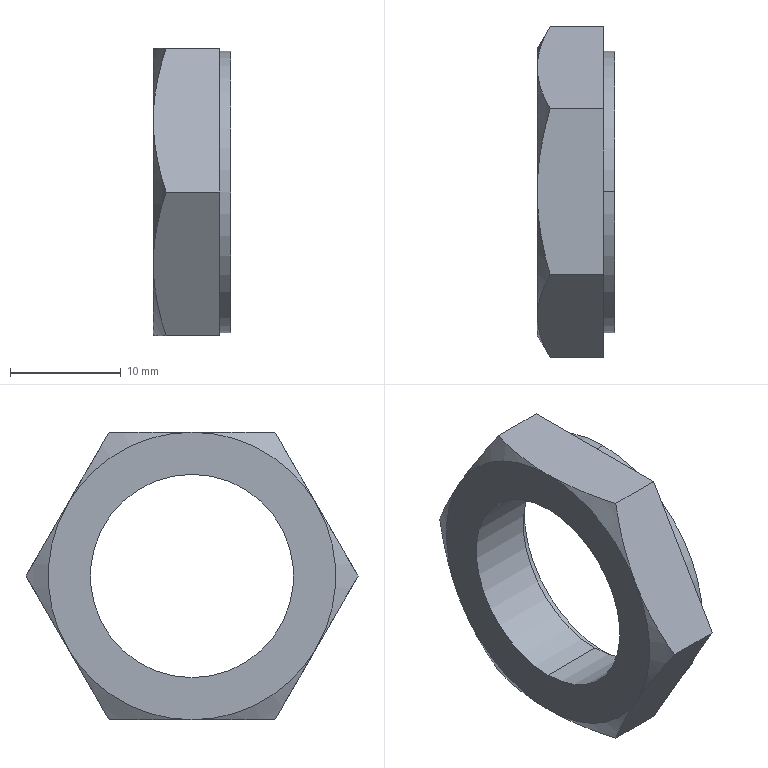Part | 1 solid | 22 faces | box 7 x 30.022 x 26 mm | volume 2098 mm3 | plane 10 | cylinder 6 | cone 6 | commonest cylinder face diameters 18.376 x2 20 x2 25.5 x2
STEP:
#1=CARTESIAN_POINT('',(7.,0.,-12.75));
#2=VERTEX_POINT('',#1);
#3=CARTESIAN_POINT('',(7.,0.,12.75));
#4=VERTEX_POINT('',#3);
#5=CARTESIAN_POINT('',(7.,0.,0.));
#6=DIRECTION('',(1.,0.,0.));
#7=DIRECTION('',(0.,0.,-1.));
#8=AXIS2_PLACEMENT_3D('',#5,#6,#7);
#9=CIRCLE('',#8,12.75);
#10=EDGE_CURVE('',#2,#4,#9,.T.);
#11=ORIENTED_EDGE('',*,*,#10,.F.);
#12=CARTESIAN_POINT('',(6.,0.,-12.75));
#13=VERTEX_POINT('',#12);
#14=CARTESIAN_POINT('',(7.,0.,-12.75));
#15=DIRECTION('',(-1.,0.,0.));
#16=VECTOR('',#15,1000.);
#17=LINE('',#14,#16);
#18=EDGE_CURVE('',#2,#13,#17,.T.);
#19=ORIENTED_EDGE('',*,*,#18,.T.);
#20=CARTESIAN_POINT('',(6.,0.,12.75));
#21=VERTEX_POINT('',#20);
#22=CARTESIAN_POINT('',(6.,0.,0.));
#23=DIRECTION('',(1.,0.,0.));
#24=DIRECTION('',(0.,0.,-1.));
#25=AXIS2_PLACEMENT_3D('',#22,#23,#24);
#26=CIRCLE('',#25,12.75);
#27=EDGE_CURVE('',#13,#21,#26,.T.);
#28=ORIENTED_EDGE('',*,*,#27,.T.);
#29=CARTESIAN_POINT('',(7.,0.,12.75));
#30=DIRECTION('',(-1.,0.,0.));
#31=VECTOR('',#30,1000.);
#32=LINE('',#29,#31);
#33=EDGE_CURVE('',#4,#21,#32,.T.);
#34=ORIENTED_EDGE('',*,*,#33,.F.);
#35=EDGE_LOOP('',(#11,#19,#28,#34));
#36=FACE_OUTER_BOUND('',#35,.T.);
#37=CARTESIAN_POINT('',(7.,0.,0.));
#38=DIRECTION('',(-1.,0.,0.));
#39=DIRECTION('',(0.,0.,1.));
#40=AXIS2_PLACEMENT_3D('',#37,#38,#39);
#41=CYLINDRICAL_SURFACE('',#40,12.75);
#42=ADVANCED_FACE('',(#36),#41,.T.);
#43=CARTESIAN_POINT('',(7.,0.,10.));
#44=VERTEX_POINT('',#43);
#45=CARTESIAN_POINT('',(7.,0.,-10.));
#46=VERTEX_POINT('',#45);
#47=CARTESIAN_POINT('',(7.,0.,0.));
#48=DIRECTION('',(1.,0.,0.));
#49=DIRECTION('',(0.,0.,-1.));
#50=AXIS2_PLACEMENT_3D('',#47,#48,#49);
#51=CIRCLE('',#50,10.);
#52=EDGE_CURVE('',#44,#46,#51,.T.);
#53=ORIENTED_EDGE('',*,*,#52,.T.);
#54=CARTESIAN_POINT('',(6.,0.,-10.));
#55=VERTEX_POINT('',#54);
#56=CARTESIAN_POINT('',(7.,0.,-10.));
#57=DIRECTION('',(-1.,0.,0.));
#58=VECTOR('',#57,1000.);
#59=LINE('',#56,#58);
#60=EDGE_CURVE('',#46,#55,#59,.T.);
#61=ORIENTED_EDGE('',*,*,#60,.T.);
#62=CARTESIAN_POINT('',(6.,0.,10.));
#63=VERTEX_POINT('',#62);
#64=CARTESIAN_POINT('',(6.,0.,0.));
#65=DIRECTION('',(-1.,0.,0.));
#66=DIRECTION('',(0.,0.,-1.));
#67=AXIS2_PLACEMENT_3D('',#64,#65,#66);
#68=CIRCLE('',#67,10.);
#69=EDGE_CURVE('',#55,#63,#68,.T.);
#70=ORIENTED_EDGE('',*,*,#69,.T.);
#71=CARTESIAN_POINT('',(7.,0.,10.));
#72=DIRECTION('',(-1.,0.,0.));
#73=VECTOR('',#72,1000.);
#74=LINE('',#71,#73);
#75=EDGE_CURVE('',#44,#63,#74,.T.);
#76=ORIENTED_EDGE('',*,*,#75,.F.);
#77=EDGE_LOOP('',(#53,#61,#70,#76));
#78=FACE_OUTER_BOUND('',#77,.T.);
#79=CARTESIAN_POINT('',(7.,0.,0.));
#80=DIRECTION('',(-1.,0.,0.));
#81=DIRECTION('',(0.,0.,1.));
#82=AXIS2_PLACEMENT_3D('',#79,#80,#81);
#83=CYLINDRICAL_SURFACE('',#82,10.);
#84=ADVANCED_FACE('',(#78),#83,.F.);
#85=CARTESIAN_POINT('',(0.,0.,9.188));
#86=VERTEX_POINT('',#85);
#87=CARTESIAN_POINT('',(0.,0.,-9.188));
#88=VERTEX_POINT('',#87);
#89=CARTESIAN_POINT('',(0.,0.,0.));
#90=DIRECTION('',(1.,0.,0.));
#91=DIRECTION('',(0.,0.,-1.));
#92=AXIS2_PLACEMENT_3D('',#89,#90,#91);
#93=CIRCLE('',#92,9.188);
#94=EDGE_CURVE('',#86,#88,#93,.T.);
#95=ORIENTED_EDGE('',*,*,#94,.F.);
#96=CARTESIAN_POINT('',(6.,0.,9.188));
#97=VERTEX_POINT('',#96);
#98=CARTESIAN_POINT('',(6.,0.,9.188));
#99=DIRECTION('',(1.,0.,0.));
#100=VECTOR('',#99,1000.);
#101=LINE('',#98,#100);
#102=EDGE_CURVE('',#86,#97,#101,.T.);
#103=ORIENTED_EDGE('',*,*,#102,.T.);
#104=CARTESIAN_POINT('',(6.,0.,-9.188));
#105=VERTEX_POINT('',#104);
#106=CARTESIAN_POINT('',(6.,0.,0.));
#107=DIRECTION('',(1.,0.,0.));
#108=DIRECTION('',(0.,0.,-1.));
#109=AXIS2_PLACEMENT_3D('',#106,#107,#108);
#110=CIRCLE('',#109,9.188);
#111=EDGE_CURVE('',#97,#105,#110,.T.);
#112=ORIENTED_EDGE('',*,*,#111,.T.);
#113=CARTESIAN_POINT('',(6.,0.,-9.188));
#114=DIRECTION('',(1.,0.,0.));
#115=VECTOR('',#114,1000.);
#116=LINE('',#113,#115);
#117=EDGE_CURVE('',#88,#105,#116,.T.);
#118=ORIENTED_EDGE('',*,*,#117,.F.);
#119=EDGE_LOOP('',(#95,#103,#112,#118));
#120=FACE_OUTER_BOUND('',#119,.T.);
#121=CARTESIAN_POINT('',(6.,0.,0.));
#122=DIRECTION('',(1.,0.,0.));
#123=DIRECTION('',(0.,0.,-1.));
#124=AXIS2_PLACEMENT_3D('',#121,#122,#123);
#125=CYLINDRICAL_SURFACE('',#124,9.188);
#126=ADVANCED_FACE('',(#120),#125,.F.);
#127=CARTESIAN_POINT('',(1.161,7.506,-13.));
#128=VERTEX_POINT('',#127);
#129=CARTESIAN_POINT('',(0.,11.258,-6.5));
#130=VERTEX_POINT('',#129);
#131=CARTESIAN_POINT('',(1.161,7.506,-13.));
#132=CARTESIAN_POINT('',(0.387,8.846,-10.678));
#133=CARTESIAN_POINT('',(0.,10.097,-8.511));
#134=CARTESIAN_POINT('',(0.,11.258,-6.5));
#135=B_SPLINE_CURVE_WITH_KNOTS('',3,(#131,#132,#133,#134),.UNSPECIFIED.,.F.,.F.,(4,4),(0.,1.),.UNSPECIFIED.);
#136=EDGE_CURVE('',#128,#130,#135,.T.);
#137=ORIENTED_EDGE('',*,*,#136,.F.);
#138=CARTESIAN_POINT('',(0.,0.,-13.));
#139=VERTEX_POINT('',#138);
#140=CARTESIAN_POINT('',(0.,0.,-13.));
#141=CARTESIAN_POINT('',(0.,2.322,-13.));
#142=CARTESIAN_POINT('',(0.387,4.824,-13.));
#143=CARTESIAN_POINT('',(1.161,7.506,-13.));
#144=B_SPLINE_CURVE_WITH_KNOTS('',3,(#140,#141,#142,#143),.UNSPECIFIED.,.F.,.F.,(4,4),(0.,1.),.UNSPECIFIED.);
#145=EDGE_CURVE('',#139,#128,#144,.T.);
#146=ORIENTED_EDGE('',*,*,#145,.F.);
#147=CARTESIAN_POINT('',(0.,0.,0.));
#148=DIRECTION('',(1.,0.,0.));
#149=DIRECTION('',(0.,0.,-1.));
#150=AXIS2_PLACEMENT_3D('',#147,#148,#149);
#151=CIRCLE('',#150,13.);
#152=EDGE_CURVE('',#139,#130,#151,.T.);
#153=ORIENTED_EDGE('',*,*,#152,.T.);
#154=EDGE_LOOP('',(#137,#146,#153));
#155=FACE_OUTER_BOUND('',#154,.T.);
#156=CARTESIAN_POINT('',(3.,0.,0.));
#157=DIRECTION('',(1.,0.,0.));
#158=DIRECTION('',(0.,0.,-1.));
#159=AXIS2_PLACEMENT_3D('',#156,#157,#158);
#160=CONICAL_SURFACE('',#159,18.196,1.047);
#161=ADVANCED_FACE('',(#155),#160,.T.);
#162=CARTESIAN_POINT('',(1.161,15.011,0.));
#163=VERTEX_POINT('',#162);
#164=CARTESIAN_POINT('',(0.,11.258,-6.5));
#165=CARTESIAN_POINT('',(0.,12.419,-4.489));
#166=CARTESIAN_POINT('',(0.387,13.67,-2.322));
#167=CARTESIAN_POINT('',(1.161,15.011,0.));
#168=B_SPLINE_CURVE_WITH_KNOTS('',3,(#164,#165,#166,#167),.UNSPECIFIED.,.F.,.F.,(4,4),(0.,1.),.UNSPECIFIED.);
#169=EDGE_CURVE('',#130,#163,#168,.T.);
#170=ORIENTED_EDGE('',*,*,#169,.F.);
#171=CARTESIAN_POINT('',(0.,11.258,6.5));
#172=VERTEX_POINT('',#171);
#173=CARTESIAN_POINT('',(0.,0.,0.));
#174=DIRECTION('',(1.,0.,0.));
#175=DIRECTION('',(0.,0.,-1.));
#176=AXIS2_PLACEMENT_3D('',#173,#174,#175);
#177=CIRCLE('',#176,13.);
#178=EDGE_CURVE('',#130,#172,#177,.T.);
#179=ORIENTED_EDGE('',*,*,#178,.T.);
#180=CARTESIAN_POINT('',(1.161,15.011,0.));
#181=CARTESIAN_POINT('',(0.387,13.67,2.322));
#182=CARTESIAN_POINT('',(0.,12.419,4.489));
#183=CARTESIAN_POINT('',(0.,11.258,6.5));
#184=B_SPLINE_CURVE_WITH_KNOTS('',3,(#180,#181,#182,#183),.UNSPECIFIED.,.F.,.F.,(4,4),(0.,1.),.UNSPECIFIED.);
#185=EDGE_CURVE('',#163,#172,#184,.T.);
#186=ORIENTED_EDGE('',*,*,#185,.F.);
#187=EDGE_LOOP('',(#170,#179,#186));
#188=FACE_OUTER_BOUND('',#187,.T.);
#189=CARTESIAN_POINT('',(3.,0.,0.));
#190=DIRECTION('',(1.,0.,0.));
#191=DIRECTION('',(0.,0.,-1.));
#192=AXIS2_PLACEMENT_3D('',#189,#190,#191);
#193=CONICAL_SURFACE('',#192,18.196,1.047);
#194=ADVANCED_FACE('',(#188),#193,.T.);
#195=CARTESIAN_POINT('',(1.161,7.506,13.));
#196=VERTEX_POINT('',#195);
#197=CARTESIAN_POINT('',(0.,11.258,6.5));
#198=CARTESIAN_POINT('',(0.,10.097,8.511));
#199=CARTESIAN_POINT('',(0.387,8.846,10.678));
#200=CARTESIAN_POINT('',(1.161,7.506,13.));
#201=B_SPLINE_CURVE_WITH_KNOTS('',3,(#197,#198,#199,#200),.UNSPECIFIED.,.F.,.F.,(4,4),(0.,1.),.UNSPECIFIED.);
#202=EDGE_CURVE('',#172,#196,#201,.T.);
#203=ORIENTED_EDGE('',*,*,#202,.F.);
#204=CARTESIAN_POINT('',(0.,0.,13.));
#205=VERTEX_POINT('',#204);
#206=CARTESIAN_POINT('',(0.,0.,0.));
#207=DIRECTION('',(1.,0.,0.));
#208=DIRECTION('',(0.,0.,-1.));
#209=AXIS2_PLACEMENT_3D('',#206,#207,#208);
#210=CIRCLE('',#209,13.);
#211=EDGE_CURVE('',#172,#205,#210,.T.);
#212=ORIENTED_EDGE('',*,*,#211,.T.);
#213=CARTESIAN_POINT('',(1.161,7.506,13.));
#214=CARTESIAN_POINT('',(0.387,4.824,13.));
#215=CARTESIAN_POINT('',(0.,2.322,13.));
#216=CARTESIAN_POINT('',(0.,0.,13.));
#217=B_SPLINE_CURVE_WITH_KNOTS('',3,(#213,#214,#215,#216),.UNSPECIFIED.,.F.,.F.,(4,4),(0.,1.),.UNSPECIFIED.);
#218=EDGE_CURVE('',#196,#205,#217,.T.);
#219=ORIENTED_EDGE('',*,*,#218,.F.);
#220=EDGE_LOOP('',(#203,#212,#219));
#221=FACE_OUTER_BOUND('',#220,.T.);
#222=CARTESIAN_POINT('',(3.,0.,0.));
#223=DIRECTION('',(1.,0.,0.));
#224=DIRECTION('',(0.,0.,-1.));
#225=AXIS2_PLACEMENT_3D('',#222,#223,#224);
#226=CONICAL_SURFACE('',#225,18.196,1.047);
#227=ADVANCED_FACE('',(#221),#226,.T.);
#228=CARTESIAN_POINT('',(1.161,-7.506,-13.));
#229=VERTEX_POINT('',#228);
#230=CARTESIAN_POINT('',(1.161,-7.506,-13.));
#231=CARTESIAN_POINT('',(0.387,-4.824,-13.));
#232=CARTESIAN_POINT('',(0.,-2.322,-13.));
#233=CARTESIAN_POINT('',(0.,0.,-13.));
#234=B_SPLINE_CURVE_WITH_KNOTS('',3,(#230,#231,#232,#233),.UNSPECIFIED.,.F.,.F.,(4,4),(0.,1.),.UNSPECIFIED.);
#235=EDGE_CURVE('',#229,#139,#234,.T.);
#236=ORIENTED_EDGE('',*,*,#235,.F.);
#237=CARTESIAN_POINT('',(0.,-11.258,-6.5));
#238=VERTEX_POINT('',#237);
#239=CARTESIAN_POINT('',(0.,-11.258,-6.5));
#240=CARTESIAN_POINT('',(0.,-10.097,-8.511));
#241=CARTESIAN_POINT('',(0.387,-8.846,-10.678));
#242=CARTESIAN_POINT('',(1.161,-7.506,-13.));
#243=B_SPLINE_CURVE_WITH_KNOTS('',3,(#239,#240,#241,#242),.UNSPECIFIED.,.F.,.F.,(4,4),(0.,1.),.UNSPECIFIED.);
#244=EDGE_CURVE('',#238,#229,#243,.T.);
#245=ORIENTED_EDGE('',*,*,#244,.F.);
#246=CARTESIAN_POINT('',(0.,0.,0.));
#247=DIRECTION('',(1.,0.,0.));
#248=DIRECTION('',(0.,0.,-1.));
#249=AXIS2_PLACEMENT_3D('',#246,#247,#248);
#250=CIRCLE('',#249,13.);
#251=EDGE_CURVE('',#238,#139,#250,.T.);
#252=ORIENTED_EDGE('',*,*,#251,.T.);
#253=EDGE_LOOP('',(#236,#245,#252));
#254=FACE_OUTER_BOUND('',#253,.T.);
#255=CARTESIAN_POINT('',(3.,0.,0.));
#256=DIRECTION('',(1.,0.,0.));
#257=DIRECTION('',(0.,0.,-1.));
#258=AXIS2_PLACEMENT_3D('',#255,#256,#257);
#259=CONICAL_SURFACE('',#258,18.196,1.047);
#260=ADVANCED_FACE('',(#254),#259,.T.);
#261=CARTESIAN_POINT('',(1.161,-7.506,13.));
#262=VERTEX_POINT('',#261);
#263=CARTESIAN_POINT('',(0.,0.,13.));
#264=CARTESIAN_POINT('',(0.,-2.322,13.));
#265=CARTESIAN_POINT('',(0.387,-4.824,13.));
#266=CARTESIAN_POINT('',(1.161,-7.506,13.));
#267=B_SPLINE_CURVE_WITH_KNOTS('',3,(#263,#264,#265,#266),.UNSPECIFIED.,.F.,.F.,(4,4),(0.,1.),.UNSPECIFIED.);
#268=EDGE_CURVE('',#205,#262,#267,.T.);
#269=ORIENTED_EDGE('',*,*,#268,.F.);
#270=CARTESIAN_POINT('',(0.,-11.258,6.5));
#271=VERTEX_POINT('',#270);
#272=CARTESIAN_POINT('',(0.,0.,0.));
#273=DIRECTION('',(1.,0.,0.));
#274=DIRECTION('',(0.,0.,-1.));
#275=AXIS2_PLACEMENT_3D('',#272,#273,#274);
#276=CIRCLE('',#275,13.);
#277=EDGE_CURVE('',#205,#271,#276,.T.);
#278=ORIENTED_EDGE('',*,*,#277,.T.);
#279=CARTESIAN_POINT('',(1.161,-7.506,13.));
#280=CARTESIAN_POINT('',(0.387,-8.846,10.678));
#281=CARTESIAN_POINT('',(0.,-10.097,8.511));
#282=CARTESIAN_POINT('',(0.,-11.258,6.5));
#283=B_SPLINE_CURVE_WITH_KNOTS('',3,(#279,#280,#281,#282),.UNSPECIFIED.,.F.,.F.,(4,4),(0.,1.),.UNSPECIFIED.);
#284=EDGE_CURVE('',#262,#271,#283,.T.);
#285=ORIENTED_EDGE('',*,*,#284,.F.);
#286=EDGE_LOOP('',(#269,#278,#285));
#287=FACE_OUTER_BOUND('',#286,.T.);
#288=CARTESIAN_POINT('',(3.,0.,0.));
#289=DIRECTION('',(1.,0.,0.));
#290=DIRECTION('',(0.,0.,-1.));
#291=AXIS2_PLACEMENT_3D('',#288,#289,#290);
#292=CONICAL_SURFACE('',#291,18.196,1.047);
#293=ADVANCED_FACE('',(#287),#292,.T.);
#294=CARTESIAN_POINT('',(6.,0.,0.));
#295=DIRECTION('',(1.,0.,0.));
#296=DIRECTION('',(0.,0.,-1.));
#297=AXIS2_PLACEMENT_3D('',#294,#295,#296);
#298=CIRCLE('',#297,9.188);
#299=EDGE_CURVE('',#105,#97,#298,.T.);
#300=ORIENTED_EDGE('',*,*,#299,.F.);
#301=ORIENTED_EDGE('',*,*,#111,.F.);
#302=EDGE_LOOP('',(#300,#301));
#303=FACE_BOUND('',#302,.T.);
#304=CARTESIAN_POINT('',(6.,0.,0.));
#305=DIRECTION('',(-1.,0.,0.));
#306=DIRECTION('',(0.,0.,-1.));
#307=AXIS2_PLACEMENT_3D('',#304,#305,#306);
#308=CIRCLE('',#307,10.);
#309=EDGE_CURVE('',#63,#55,#308,.T.);
#310=ORIENTED_EDGE('',*,*,#309,.F.);
#311=ORIENTED_EDGE('',*,*,#69,.F.);
#312=EDGE_LOOP('',(#310,#311));
#313=FACE_OUTER_BOUND('',#312,.T.);
#314=CARTESIAN_POINT('',(6.,9.188,0.));
#315=DIRECTION('',(1.,0.,0.));
#316=DIRECTION('',(0.,1.,0.));
#317=AXIS2_PLACEMENT_3D('',#314,#315,#316);
#318=PLANE('',#317);
#319=ADVANCED_FACE('',(#303,#313),#318,.T.);
#320=CARTESIAN_POINT('',(0.,0.,0.));
#321=DIRECTION('',(1.,0.,0.));
#322=DIRECTION('',(0.,0.,-1.));
#323=AXIS2_PLACEMENT_3D('',#320,#321,#322);
#324=CIRCLE('',#323,9.188);
#325=EDGE_CURVE('',#88,#86,#324,.T.);
#326=ORIENTED_EDGE('',*,*,#325,.T.);
#327=ORIENTED_EDGE('',*,*,#94,.T.);
#328=EDGE_LOOP('',(#326,#327));
#329=FACE_BOUND('',#328,.T.);
#330=ORIENTED_EDGE('',*,*,#152,.F.);
#331=ORIENTED_EDGE('',*,*,#251,.F.);
#332=CARTESIAN_POINT('',(0.,0.,0.));
#333=DIRECTION('',(1.,0.,0.));
#334=DIRECTION('',(0.,0.,-1.));
#335=AXIS2_PLACEMENT_3D('',#332,#333,#334);
#336=CIRCLE('',#335,13.);
#337=EDGE_CURVE('',#271,#238,#336,.T.);
#338=ORIENTED_EDGE('',*,*,#337,.F.);
#339=ORIENTED_EDGE('',*,*,#277,.F.);
#340=ORIENTED_EDGE('',*,*,#211,.F.);
#341=ORIENTED_EDGE('',*,*,#178,.F.);
#342=EDGE_LOOP('',(#330,#331,#338,#339,#340,#341));
#343=FACE_OUTER_BOUND('',#342,.T.);
#344=CARTESIAN_POINT('',(0.,13.,0.));
#345=DIRECTION('',(-1.,0.,0.));
#346=DIRECTION('',(0.,0.,1.));
#347=AXIS2_PLACEMENT_3D('',#344,#345,#346);
#348=PLANE('',#347);
#349=ADVANCED_FACE('',(#329,#343),#348,.T.);
#350=ORIENTED_EDGE('',*,*,#102,.F.);
#351=ORIENTED_EDGE('',*,*,#325,.F.);
#352=ORIENTED_EDGE('',*,*,#117,.T.);
#353=ORIENTED_EDGE('',*,*,#299,.T.);
#354=EDGE_LOOP('',(#350,#351,#352,#353));
#355=FACE_OUTER_BOUND('',#354,.T.);
#356=CARTESIAN_POINT('',(6.,0.,0.));
#357=DIRECTION('',(1.,0.,0.));
#358=DIRECTION('',(0.,0.,-1.));
#359=AXIS2_PLACEMENT_3D('',#356,#357,#358);
#360=CYLINDRICAL_SURFACE('',#359,9.188);
#361=ADVANCED_FACE('',(#355),#360,.F.);
#362=CARTESIAN_POINT('',(6.,-7.506,13.));
#363=VERTEX_POINT('',#362);
#364=CARTESIAN_POINT('',(6.,7.506,13.));
#365=VERTEX_POINT('',#364);
#366=CARTESIAN_POINT('',(6.,9.188,13.));
#367=DIRECTION('',(0.,1.,0.));
#368=VECTOR('',#367,1000.);
#369=LINE('',#366,#368);
#370=EDGE_CURVE('',#363,#365,#369,.T.);
#371=ORIENTED_EDGE('',*,*,#370,.F.);
#372=CARTESIAN_POINT('',(6.,-15.011,0.));
#373=VERTEX_POINT('',#372);
#374=CARTESIAN_POINT('',(6.,-8.961,10.479));
#375=DIRECTION('',(0.,0.5,0.866));
#376=VECTOR('',#375,1000.);
#377=LINE('',#374,#376);
#378=EDGE_CURVE('',#373,#363,#377,.T.);
#379=ORIENTED_EDGE('',*,*,#378,.F.);
#380=CARTESIAN_POINT('',(6.,-7.506,-13.));
#381=VERTEX_POINT('',#380);
#382=CARTESIAN_POINT('',(6.,-8.961,-10.479));
#383=DIRECTION('',(0.,-0.5,0.866));
#384=VECTOR('',#383,1000.);
#385=LINE('',#382,#384);
#386=EDGE_CURVE('',#381,#373,#385,.T.);
#387=ORIENTED_EDGE('',*,*,#386,.F.);
#388=CARTESIAN_POINT('',(6.,7.506,-13.));
#389=VERTEX_POINT('',#388);
#390=CARTESIAN_POINT('',(6.,9.188,-13.));
#391=DIRECTION('',(0.,-1.,0.));
#392=VECTOR('',#391,1000.);
#393=LINE('',#390,#392);
#394=EDGE_CURVE('',#389,#381,#393,.T.);
#395=ORIENTED_EDGE('',*,*,#394,.F.);
#396=CARTESIAN_POINT('',(6.,15.011,0.));
#397=VERTEX_POINT('',#396);
#398=CARTESIAN_POINT('',(6.,13.555,-2.521));
#399=DIRECTION('',(0.,-0.5,-0.866));
#400=VECTOR('',#399,1000.);
#401=LINE('',#398,#400);
#402=EDGE_CURVE('',#397,#389,#401,.T.);
#403=ORIENTED_EDGE('',*,*,#402,.F.);
#404=CARTESIAN_POINT('',(6.,13.555,2.521));
#405=DIRECTION('',(0.,0.5,-0.866));
#406=VECTOR('',#405,1000.);
#407=LINE('',#404,#406);
#408=EDGE_CURVE('',#365,#397,#407,.T.);
#409=ORIENTED_EDGE('',*,*,#408,.F.);
#410=EDGE_LOOP('',(#371,#379,#387,#395,#403,#409));
#411=FACE_OUTER_BOUND('',#410,.T.);
#412=CARTESIAN_POINT('',(6.,0.,0.));
#413=DIRECTION('',(1.,0.,0.));
#414=DIRECTION('',(0.,0.,-1.));
#415=AXIS2_PLACEMENT_3D('',#412,#413,#414);
#416=CIRCLE('',#415,12.75);
#417=EDGE_CURVE('',#21,#13,#416,.T.);
#418=ORIENTED_EDGE('',*,*,#417,.F.);
#419=ORIENTED_EDGE('',*,*,#27,.F.);
#420=EDGE_LOOP('',(#418,#419));
#421=FACE_BOUND('',#420,.T.);
#422=CARTESIAN_POINT('',(6.,9.188,0.));
#423=DIRECTION('',(1.,0.,0.));
#424=DIRECTION('',(0.,1.,0.));
#425=AXIS2_PLACEMENT_3D('',#422,#423,#424);
#426=PLANE('',#425);
#427=ADVANCED_FACE('',(#411,#421),#426,.T.);
#428=CARTESIAN_POINT('',(1.161,-15.011,0.));
#429=VERTEX_POINT('',#428);
#430=CARTESIAN_POINT('',(1.161,-15.011,0.));
#431=CARTESIAN_POINT('',(0.387,-13.67,-2.322));
#432=CARTESIAN_POINT('',(0.,-12.419,-4.489));
#433=CARTESIAN_POINT('',(0.,-11.258,-6.5));
#434=B_SPLINE_CURVE_WITH_KNOTS('',3,(#430,#431,#432,#433),.UNSPECIFIED.,.F.,.F.,(4,4),(0.,1.),.UNSPECIFIED.);
#435=EDGE_CURVE('',#429,#238,#434,.T.);
#436=ORIENTED_EDGE('',*,*,#435,.F.);
#437=CARTESIAN_POINT('',(0.,-11.258,6.5));
#438=CARTESIAN_POINT('',(0.,-12.419,4.489));
#439=CARTESIAN_POINT('',(0.387,-13.67,2.322));
#440=CARTESIAN_POINT('',(1.161,-15.011,0.));
#441=B_SPLINE_CURVE_WITH_KNOTS('',3,(#437,#438,#439,#440),.UNSPECIFIED.,.F.,.F.,(4,4),(0.,1.),.UNSPECIFIED.);
#442=EDGE_CURVE('',#271,#429,#441,.T.);
#443=ORIENTED_EDGE('',*,*,#442,.F.);
#444=ORIENTED_EDGE('',*,*,#337,.T.);
#445=EDGE_LOOP('',(#436,#443,#444));
#446=FACE_OUTER_BOUND('',#445,.T.);
#447=CARTESIAN_POINT('',(3.,0.,0.));
#448=DIRECTION('',(1.,0.,0.));
#449=DIRECTION('',(0.,0.,-1.));
#450=AXIS2_PLACEMENT_3D('',#447,#448,#449);
#451=CONICAL_SURFACE('',#450,18.196,1.047);
#452=ADVANCED_FACE('',(#446),#451,.T.);
#453=ORIENTED_EDGE('',*,*,#60,.F.);
#454=CARTESIAN_POINT('',(7.,0.,0.));
#455=DIRECTION('',(1.,0.,0.));
#456=DIRECTION('',(0.,0.,-1.));
#457=AXIS2_PLACEMENT_3D('',#454,#455,#456);
#458=CIRCLE('',#457,10.);
#459=EDGE_CURVE('',#46,#44,#458,.T.);
#460=ORIENTED_EDGE('',*,*,#459,.T.);
#461=ORIENTED_EDGE('',*,*,#75,.T.);
#462=ORIENTED_EDGE('',*,*,#309,.T.);
#463=EDGE_LOOP('',(#453,#460,#461,#462));
#464=FACE_OUTER_BOUND('',#463,.T.);
#465=CARTESIAN_POINT('',(7.,0.,0.));
#466=DIRECTION('',(-1.,0.,0.));
#467=DIRECTION('',(0.,0.,1.));
#468=AXIS2_PLACEMENT_3D('',#465,#466,#467);
#469=CYLINDRICAL_SURFACE('',#468,10.);
#470=ADVANCED_FACE('',(#464),#469,.F.);
#471=ORIENTED_EDGE('',*,*,#18,.F.);
#472=CARTESIAN_POINT('',(7.,0.,0.));
#473=DIRECTION('',(1.,0.,0.));
#474=DIRECTION('',(0.,0.,-1.));
#475=AXIS2_PLACEMENT_3D('',#472,#473,#474);
#476=CIRCLE('',#475,12.75);
#477=EDGE_CURVE('',#4,#2,#476,.T.);
#478=ORIENTED_EDGE('',*,*,#477,.F.);
#479=ORIENTED_EDGE('',*,*,#33,.T.);
#480=ORIENTED_EDGE('',*,*,#417,.T.);
#481=EDGE_LOOP('',(#471,#478,#479,#480));
#482=FACE_OUTER_BOUND('',#481,.T.);
#483=CARTESIAN_POINT('',(7.,0.,0.));
#484=DIRECTION('',(-1.,0.,0.));
#485=DIRECTION('',(0.,0.,1.));
#486=AXIS2_PLACEMENT_3D('',#483,#484,#485);
#487=CYLINDRICAL_SURFACE('',#486,12.75);
#488=ADVANCED_FACE('',(#482),#487,.T.);
#489=ORIENTED_EDGE('',*,*,#52,.F.);
#490=ORIENTED_EDGE('',*,*,#459,.F.);
#491=EDGE_LOOP('',(#489,#490));
#492=FACE_BOUND('',#491,.T.);
#493=ORIENTED_EDGE('',*,*,#477,.T.);
#494=ORIENTED_EDGE('',*,*,#10,.T.);
#495=EDGE_LOOP('',(#493,#494));
#496=FACE_OUTER_BOUND('',#495,.T.);
#497=CARTESIAN_POINT('',(7.,0.,0.));
#498=DIRECTION('',(1.,0.,0.));
#499=DIRECTION('',(0.,1.,0.));
#500=AXIS2_PLACEMENT_3D('',#497,#498,#499);
#501=PLANE('',#500);
#502=ADVANCED_FACE('',(#492,#496),#501,.T.);
#503=ORIENTED_EDGE('',*,*,#370,.T.);
#504=CARTESIAN_POINT('',(7.,7.506,13.));
#505=DIRECTION('',(-1.,0.,0.));
#506=VECTOR('',#505,1000.);
#507=LINE('',#504,#506);
#508=EDGE_CURVE('',#365,#196,#507,.T.);
#509=ORIENTED_EDGE('',*,*,#508,.T.);
#510=ORIENTED_EDGE('',*,*,#218,.T.);
#511=ORIENTED_EDGE('',*,*,#268,.T.);
#512=CARTESIAN_POINT('',(7.,-7.506,13.));
#513=DIRECTION('',(-1.,0.,0.));
#514=VECTOR('',#513,1000.);
#515=LINE('',#512,#514);
#516=EDGE_CURVE('',#363,#262,#515,.T.);
#517=ORIENTED_EDGE('',*,*,#516,.F.);
#518=EDGE_LOOP('',(#503,#509,#510,#511,#517));
#519=FACE_OUTER_BOUND('',#518,.T.);
#520=CARTESIAN_POINT('',(7.,7.506,13.));
#521=DIRECTION('',(0.,0.,-1.));
#522=DIRECTION('',(0.,-1.,0.));
#523=AXIS2_PLACEMENT_3D('',#520,#521,#522);
#524=PLANE('',#523);
#525=ADVANCED_FACE('',(#519),#524,.F.);
#526=ORIENTED_EDGE('',*,*,#408,.T.);
#527=CARTESIAN_POINT('',(7.,15.011,0.));
#528=DIRECTION('',(-1.,0.,0.));
#529=VECTOR('',#528,1000.);
#530=LINE('',#527,#529);
#531=EDGE_CURVE('',#397,#163,#530,.T.);
#532=ORIENTED_EDGE('',*,*,#531,.T.);
#533=ORIENTED_EDGE('',*,*,#185,.T.);
#534=ORIENTED_EDGE('',*,*,#202,.T.);
#535=ORIENTED_EDGE('',*,*,#508,.F.);
#536=EDGE_LOOP('',(#526,#532,#533,#534,#535));
#537=FACE_OUTER_BOUND('',#536,.T.);
#538=CARTESIAN_POINT('',(7.,15.011,0.));
#539=DIRECTION('',(0.,-0.866,-0.5));
#540=DIRECTION('',(0.,0.5,-0.866));
#541=AXIS2_PLACEMENT_3D('',#538,#539,#540);
#542=PLANE('',#541);
#543=ADVANCED_FACE('',(#537),#542,.F.);
#544=ORIENTED_EDGE('',*,*,#402,.T.);
#545=CARTESIAN_POINT('',(7.,7.506,-13.));
#546=DIRECTION('',(-1.,0.,0.));
#547=VECTOR('',#546,1000.);
#548=LINE('',#545,#547);
#549=EDGE_CURVE('',#389,#128,#548,.T.);
#550=ORIENTED_EDGE('',*,*,#549,.T.);
#551=ORIENTED_EDGE('',*,*,#136,.T.);
#552=ORIENTED_EDGE('',*,*,#169,.T.);
#553=ORIENTED_EDGE('',*,*,#531,.F.);
#554=EDGE_LOOP('',(#544,#550,#551,#552,#553));
#555=FACE_OUTER_BOUND('',#554,.T.);
#556=CARTESIAN_POINT('',(7.,7.506,-13.));
#557=DIRECTION('',(0.,-0.866,0.5));
#558=DIRECTION('',(-1.,0.,0.));
#559=AXIS2_PLACEMENT_3D('',#556,#557,#558);
#560=PLANE('',#559);
#561=ADVANCED_FACE('',(#555),#560,.F.);
#562=ORIENTED_EDGE('',*,*,#394,.T.);
#563=CARTESIAN_POINT('',(7.,-7.506,-13.));
#564=DIRECTION('',(-1.,0.,0.));
#565=VECTOR('',#564,1000.);
#566=LINE('',#563,#565);
#567=EDGE_CURVE('',#381,#229,#566,.T.);
#568=ORIENTED_EDGE('',*,*,#567,.T.);
#569=ORIENTED_EDGE('',*,*,#235,.T.);
#570=ORIENTED_EDGE('',*,*,#145,.T.);
#571=ORIENTED_EDGE('',*,*,#549,.F.);
#572=EDGE_LOOP('',(#562,#568,#569,#570,#571));
#573=FACE_OUTER_BOUND('',#572,.T.);
#574=CARTESIAN_POINT('',(7.,-7.506,-13.));
#575=DIRECTION('',(0.,0.,1.));
#576=DIRECTION('',(1.,0.,0.));
#577=AXIS2_PLACEMENT_3D('',#574,#575,#576);
#578=PLANE('',#577);
#579=ADVANCED_FACE('',(#573),#578,.F.);
#580=ORIENTED_EDGE('',*,*,#386,.T.);
#581=CARTESIAN_POINT('',(7.,-15.011,0.));
#582=DIRECTION('',(-1.,0.,0.));
#583=VECTOR('',#582,1000.);
#584=LINE('',#581,#583);
#585=EDGE_CURVE('',#373,#429,#584,.T.);
#586=ORIENTED_EDGE('',*,*,#585,.T.);
#587=ORIENTED_EDGE('',*,*,#435,.T.);
#588=ORIENTED_EDGE('',*,*,#244,.T.);
#589=ORIENTED_EDGE('',*,*,#567,.F.);
#590=EDGE_LOOP('',(#580,#586,#587,#588,#589));
#591=FACE_OUTER_BOUND('',#590,.T.);
#592=CARTESIAN_POINT('',(7.,-15.011,0.));
#593=DIRECTION('',(0.,0.866,0.5));
#594=DIRECTION('',(1.,0.,0.));
#595=AXIS2_PLACEMENT_3D('',#592,#593,#594);
#596=PLANE('',#595);
#597=ADVANCED_FACE('',(#591),#596,.F.);
#598=ORIENTED_EDGE('',*,*,#378,.T.);
#599=ORIENTED_EDGE('',*,*,#516,.T.);
#600=ORIENTED_EDGE('',*,*,#284,.T.);
#601=ORIENTED_EDGE('',*,*,#442,.T.);
#602=ORIENTED_EDGE('',*,*,#585,.F.);
#603=EDGE_LOOP('',(#598,#599,#600,#601,#602));
#604=FACE_OUTER_BOUND('',#603,.T.);
#605=CARTESIAN_POINT('',(7.,-7.506,13.));
#606=DIRECTION('',(0.,0.866,-0.5));
#607=DIRECTION('',(-1.,0.,0.));
#608=AXIS2_PLACEMENT_3D('',#605,#606,#607);
#609=PLANE('',#608);
#610=ADVANCED_FACE('',(#604),#609,.F.);
#611=CLOSED_SHELL('',(#42,#84,#126,#161,#194,#227,#260,#293,#319,#349,#361,#427,#452,#470,#488,#502,#525,#543,#561,#579,#597,#610));
#612=MANIFOLD_SOLID_BREP('',#611);
#613=CARTESIAN_POINT('',(0.,0.,0.));
#614=DIRECTION('',(0.,0.,1.));
#615=DIRECTION('',(1.,0.,0.));
#616=AXIS2_PLACEMENT_3D('',#613,#614,#615);
#617=(LENGTH_UNIT()NAMED_UNIT(*)SI_UNIT(.MILLI.,.METRE.));
#618=UNCERTAINTY_MEASURE_WITH_UNIT(LENGTH_MEASURE(0.00001),#617,'','');
#619=(NAMED_UNIT(*)PLANE_ANGLE_UNIT()SI_UNIT($,.RADIAN.));
#620=(NAMED_UNIT(*)SI_UNIT($,.STERADIAN.)SOLID_ANGLE_UNIT());
#621=(GEOMETRIC_REPRESENTATION_CONTEXT(3)GLOBAL_UNCERTAINTY_ASSIGNED_CONTEXT((#618))GLOBAL_UNIT_ASSIGNED_CONTEXT((#617,#619,#620))REPRESENTATION_CONTEXT('',''));
#622=ADVANCED_BREP_SHAPE_REPRESENTATION('',(#612,#616),#621);